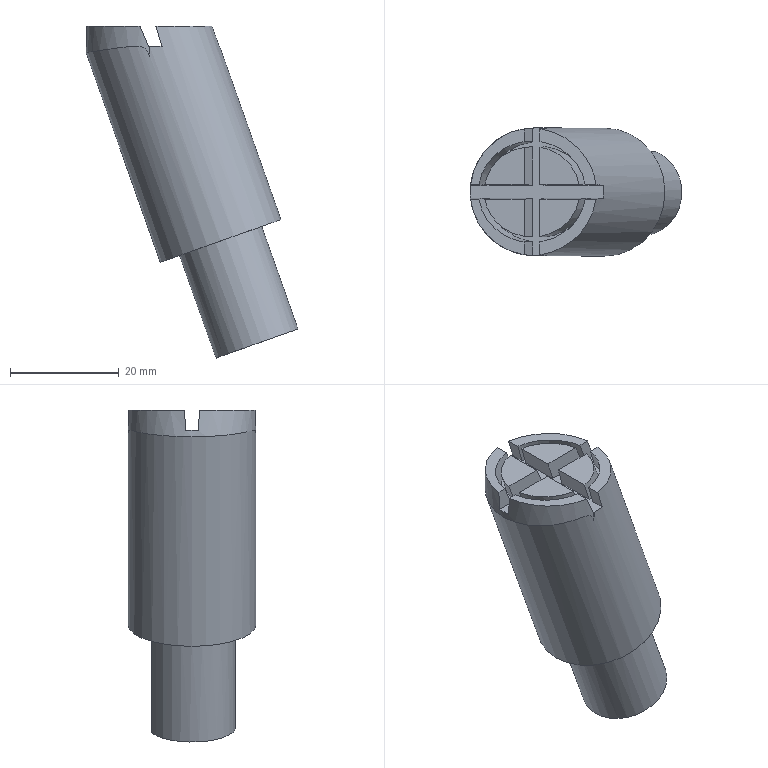Part | STEP file | SLIDE1-INSERT2_id638_x_t | 1 solid | 41 faces | box 38.941 x 23.516 x 61.041 mm | volume 21493 mm3 | plane 30 | spline 8 | cylinder 3 | commonest cylinder face diameters 16 x1 23.442 x1 23.516 x1